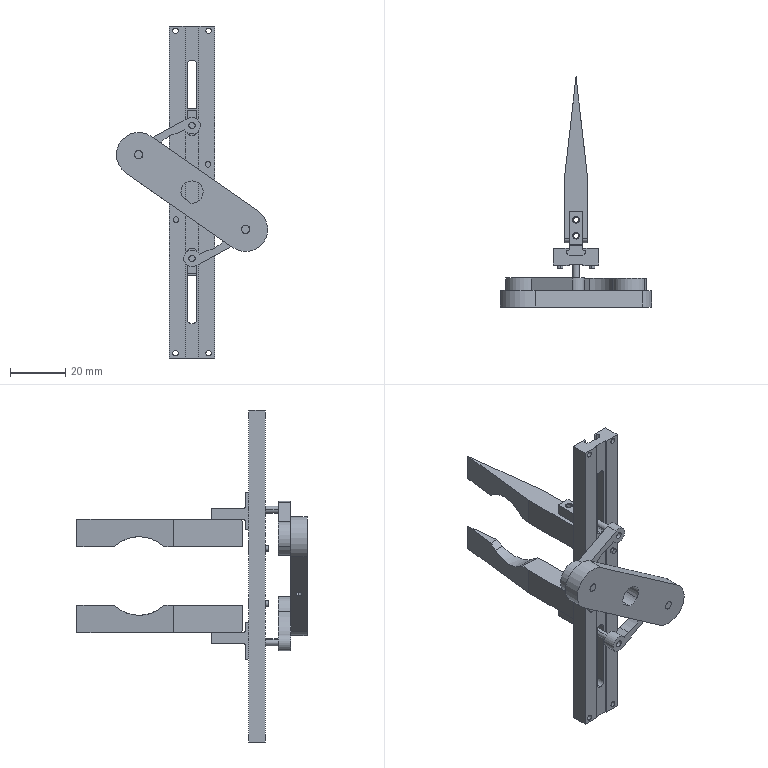Part | SolidWorks | features Cut 1, MirrorCompFeat 1 | 16 solids | 276 faces | box 54.684 x 83.216 x 120 mm | volume 23441 mm3 | cylinder 134 | plane 126 | cone 16 | commonest cylinder face diameters 2 x26 3.3 x16 1.5 x12 1.95 x8 2.013 x8 2.5 x8